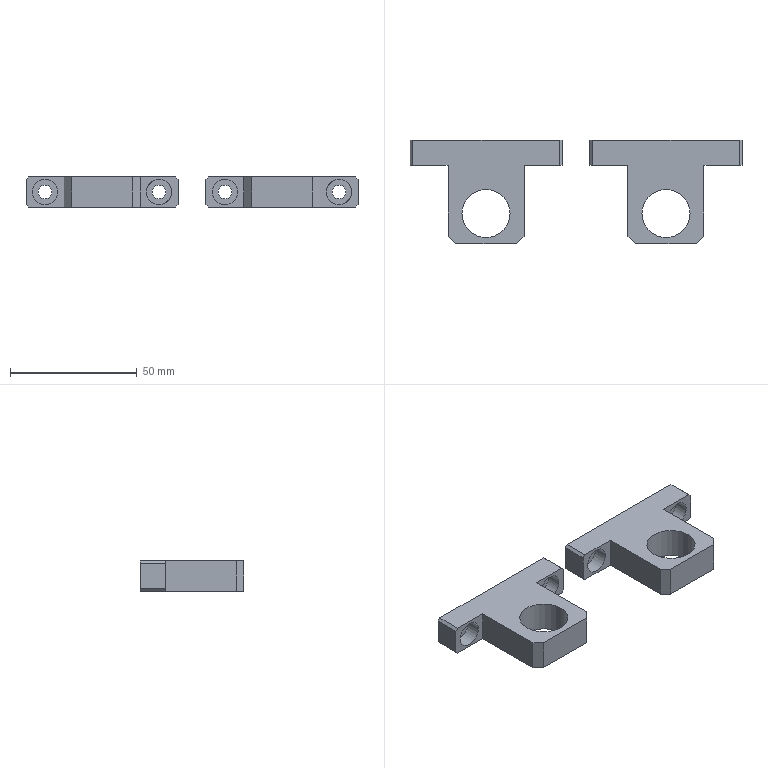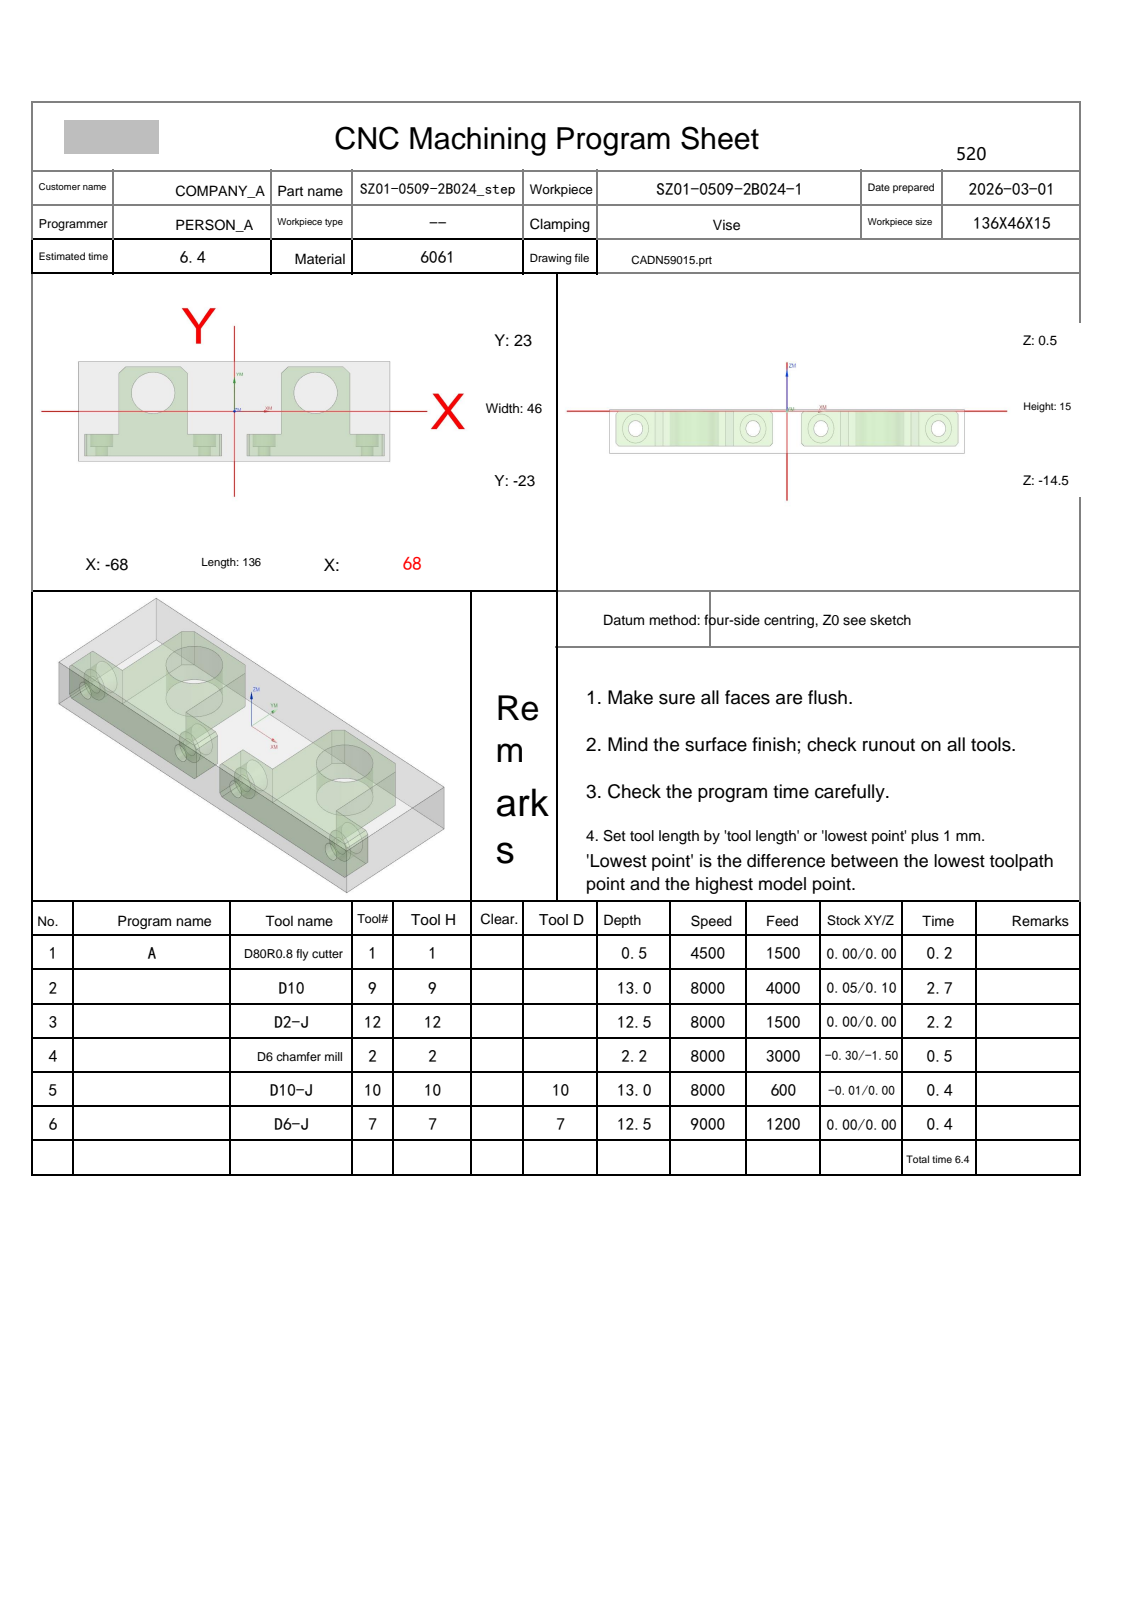NC program | NX | posted by the shop | part box 131 x 41 x 12 mm
Lines 1 to 32 of 8452:
%
O0001
(Machine time: 7.50 MIN)
(===Total Tool:6===)
(T1=D80R0.8 fly cutter D=80.  R=0.8  D-  H01 Z=-0.   )
(T9=D10     D=10.  R=0.   D-  H09 Z=-12.5 )
(T12=D2-J   D=2.   R=0.   D-  H12 Z=-12.  )
(T2=D6 chamfer mill   D=6.   R=0.   D-  H02 Z=-1.7  )
(T10=D10-J  D=10.  R=0.   D10 H10 Z=-12.5 )
(T7=D6-J    D=6.   R=0.   D7  H07 Z=-12.  )
G80 G90 G17 G49 G40
G91 G28 Z0
M01
N1 T01 M06
(D80R0.8 fly cutter  D=80. R=0.8 H=01 ce=0.00 di=0.00)
G00 G90 G54 X110.5 Y0.0 M03 S4500
G43 H01 Z50.
M08
Z2.
G01 Z0.0 F1500.
X105.5
X-105.5
X-110.5
Z2.
G00 Z50.
G91 G28 Z0.0
M05
M09
G91 G28 Z0.0
M01